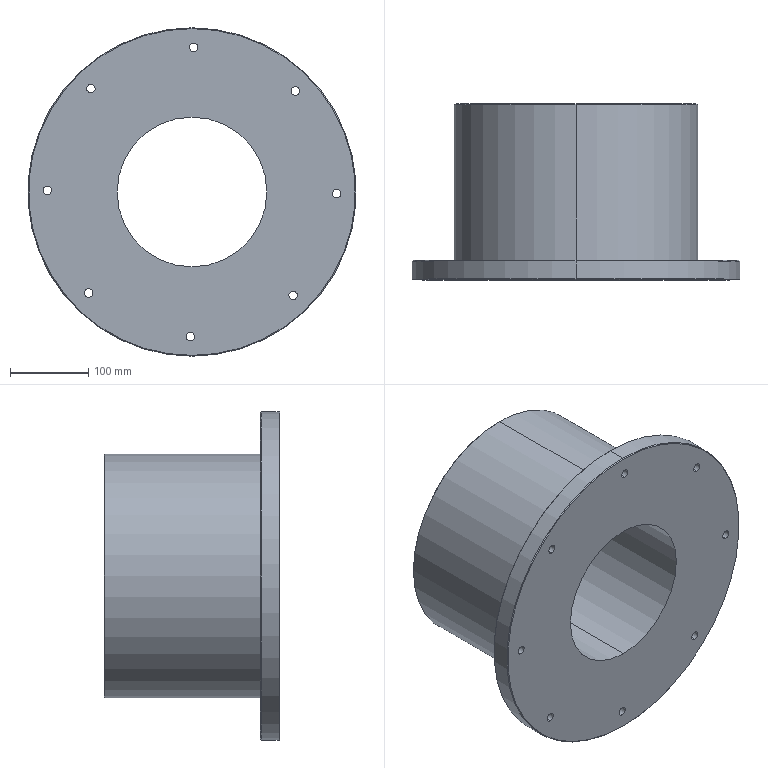Part | SolidWorks | features ICE 3, Chamfer 1, CirPattern 1, Extrusion 1, HoleWzd 1 | 1 solid | 79 faces | box 420 x 225 x 420 mm | volume 6770057 mm3 | cylinder 42 | cone 24 | plane 13 | commonest cylinder face diameters 11 x16 18 x16 191.64 x2 211.64 x2 281.64 x2 311.64 x2